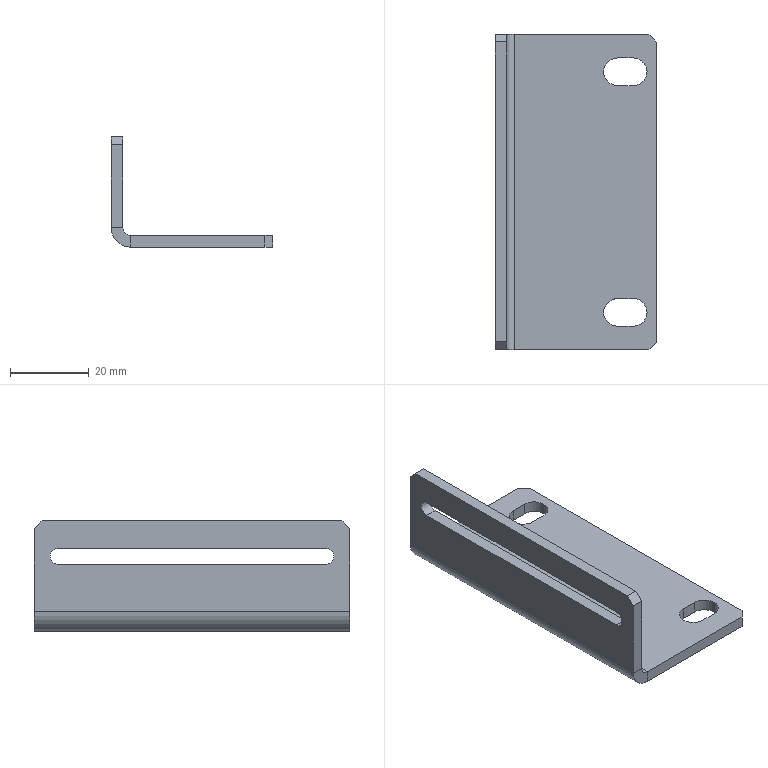Part | NX | features BREP 1 | 1 solid | 32 faces | box 41 x 80 x 28 mm | volume 14203 mm3 | plane 22 | cylinder 10 | commonest cylinder face diameters 7 x6 4 x3 10 x1
STEP:
#1=CARTESIAN_POINT('',(-2.,40.,-3.));
#2=VERTEX_POINT('',#1);
#3=CARTESIAN_POINT('',(0.,38.,-3.));
#4=VERTEX_POINT('',#3);
#5=CARTESIAN_POINT('',(0.,38.,-3.));
#6=DIRECTION('',(0.7071,-0.7071,0.));
#7=VECTOR('',#6,1000.);
#8=LINE('',#5,#7);
#9=EDGE_CURVE('',#2,#4,#8,.T.);
#10=ORIENTED_EDGE('',*,*,#9,.F.);
#11=CARTESIAN_POINT('',(-2.,40.,0.));
#12=VERTEX_POINT('',#11);
#13=CARTESIAN_POINT('',(-2.,40.,-3.));
#14=DIRECTION('',(0.,0.,-1.));
#15=VECTOR('',#14,1000.);
#16=LINE('',#13,#15);
#17=EDGE_CURVE('',#12,#2,#16,.T.);
#18=ORIENTED_EDGE('',*,*,#17,.F.);
#19=CARTESIAN_POINT('',(0.,38.,0.));
#20=VERTEX_POINT('',#19);
#21=CARTESIAN_POINT('',(-1.,39.,0.));
#22=DIRECTION('',(-0.7071,0.7071,0.));
#23=VECTOR('',#22,1000.);
#24=LINE('',#21,#23);
#25=EDGE_CURVE('',#20,#12,#24,.T.);
#26=ORIENTED_EDGE('',*,*,#25,.F.);
#27=CARTESIAN_POINT('',(0.,38.,0.));
#28=DIRECTION('',(0.,0.,1.));
#29=VECTOR('',#28,1000.);
#30=LINE('',#27,#29);
#31=EDGE_CURVE('',#4,#20,#30,.T.);
#32=ORIENTED_EDGE('',*,*,#31,.F.);
#33=EDGE_LOOP('',(#10,#18,#26,#32));
#34=FACE_BOUND('',#33,.T.);
#35=CARTESIAN_POINT('',(0.,38.,-3.));
#36=DIRECTION('',(0.7071,0.7071,0.));
#37=DIRECTION('',(0.,0.,-1.));
#38=AXIS2_PLACEMENT_3D('',#35,#36,#37);
#39=PLANE('',#38);
#40=ADVANCED_FACE('',(#34),#39,.T.);
#41=CARTESIAN_POINT('',(-38.,40.,23.));
#42=VERTEX_POINT('',#41);
#43=CARTESIAN_POINT('',(-38.,38.,25.));
#44=VERTEX_POINT('',#43);
#45=CARTESIAN_POINT('',(-38.,51.5,11.5));
#46=DIRECTION('',(0.,-0.7071,0.7071));
#47=VECTOR('',#46,1000.);
#48=LINE('',#45,#47);
#49=EDGE_CURVE('',#42,#44,#48,.T.);
#50=ORIENTED_EDGE('',*,*,#49,.F.);
#51=CARTESIAN_POINT('',(-41.,40.,23.));
#52=VERTEX_POINT('',#51);
#53=CARTESIAN_POINT('',(-36.,40.,23.));
#54=DIRECTION('',(1.,0.,0.));
#55=VECTOR('',#54,1000.);
#56=LINE('',#53,#55);
#57=EDGE_CURVE('',#52,#42,#56,.T.);
#58=ORIENTED_EDGE('',*,*,#57,.F.);
#59=CARTESIAN_POINT('',(-41.,38.,25.));
#60=VERTEX_POINT('',#59);
#61=CARTESIAN_POINT('',(-41.,38.,25.));
#62=DIRECTION('',(0.,0.7071,-0.7071));
#63=VECTOR('',#62,1000.);
#64=LINE('',#61,#63);
#65=EDGE_CURVE('',#60,#52,#64,.T.);
#66=ORIENTED_EDGE('',*,*,#65,.F.);
#67=CARTESIAN_POINT('',(-38.,38.,25.));
#68=DIRECTION('',(-1.,0.,0.));
#69=VECTOR('',#68,1000.);
#70=LINE('',#67,#69);
#71=EDGE_CURVE('',#44,#60,#70,.T.);
#72=ORIENTED_EDGE('',*,*,#71,.F.);
#73=EDGE_LOOP('',(#50,#58,#66,#72));
#74=FACE_BOUND('',#73,.T.);
#75=CARTESIAN_POINT('',(-38.,38.,25.));
#76=DIRECTION('',(0.,-0.7071,-0.7071));
#77=DIRECTION('',(-1.,0.,0.));
#78=AXIS2_PLACEMENT_3D('',#75,#76,#77);
#79=PLANE('',#78);
#80=ADVANCED_FACE('',(#74),#79,.F.);
#81=CARTESIAN_POINT('',(0.,-38.,-3.));
#82=VERTEX_POINT('',#81);
#83=CARTESIAN_POINT('',(-2.,-40.,-3.));
#84=VERTEX_POINT('',#83);
#85=CARTESIAN_POINT('',(-2.,-40.,-3.));
#86=DIRECTION('',(-0.7071,-0.7071,0.));
#87=VECTOR('',#86,1000.);
#88=LINE('',#85,#87);
#89=EDGE_CURVE('',#82,#84,#88,.T.);
#90=ORIENTED_EDGE('',*,*,#89,.F.);
#91=CARTESIAN_POINT('',(0.,-38.,0.));
#92=VERTEX_POINT('',#91);
#93=CARTESIAN_POINT('',(0.,-38.,-3.));
#94=DIRECTION('',(0.,0.,-1.));
#95=VECTOR('',#94,1000.);
#96=LINE('',#93,#95);
#97=EDGE_CURVE('',#92,#82,#96,.T.);
#98=ORIENTED_EDGE('',*,*,#97,.F.);
#99=CARTESIAN_POINT('',(-2.,-40.,0.));
#100=VERTEX_POINT('',#99);
#101=CARTESIAN_POINT('',(39.,1.,0.));
#102=DIRECTION('',(0.7071,0.7071,0.));
#103=VECTOR('',#102,1000.);
#104=LINE('',#101,#103);
#105=EDGE_CURVE('',#100,#92,#104,.T.);
#106=ORIENTED_EDGE('',*,*,#105,.F.);
#107=CARTESIAN_POINT('',(-2.,-40.,2.));
#108=DIRECTION('',(0.,0.,1.));
#109=VECTOR('',#108,1000.);
#110=LINE('',#107,#109);
#111=EDGE_CURVE('',#84,#100,#110,.T.);
#112=ORIENTED_EDGE('',*,*,#111,.F.);
#113=EDGE_LOOP('',(#90,#98,#106,#112));
#114=FACE_BOUND('',#113,.T.);
#115=CARTESIAN_POINT('',(-2.,-40.,2.));
#116=DIRECTION('',(-0.7071,0.7071,0.));
#117=DIRECTION('',(0.,0.,1.));
#118=AXIS2_PLACEMENT_3D('',#115,#116,#117);
#119=PLANE('',#118);
#120=ADVANCED_FACE('',(#114),#119,.F.);
#121=CARTESIAN_POINT('',(-38.,-38.,25.));
#122=VERTEX_POINT('',#121);
#123=CARTESIAN_POINT('',(-38.,-40.,23.));
#124=VERTEX_POINT('',#123);
#125=CARTESIAN_POINT('',(-38.,-11.5,51.5));
#126=DIRECTION('',(0.,-0.7071,-0.7071));
#127=VECTOR('',#126,1000.);
#128=LINE('',#125,#127);
#129=EDGE_CURVE('',#122,#124,#128,.T.);
#130=ORIENTED_EDGE('',*,*,#129,.F.);
#131=CARTESIAN_POINT('',(-41.,-38.,25.));
#132=VERTEX_POINT('',#131);
#133=CARTESIAN_POINT('',(-38.,-38.,25.));
#134=DIRECTION('',(1.,0.,0.));
#135=VECTOR('',#134,1000.);
#136=LINE('',#133,#135);
#137=EDGE_CURVE('',#132,#122,#136,.T.);
#138=ORIENTED_EDGE('',*,*,#137,.F.);
#139=CARTESIAN_POINT('',(-41.,-40.,23.));
#140=VERTEX_POINT('',#139);
#141=CARTESIAN_POINT('',(-41.,-40.,23.));
#142=DIRECTION('',(0.,0.7071,0.7071));
#143=VECTOR('',#142,1000.);
#144=LINE('',#141,#143);
#145=EDGE_CURVE('',#140,#132,#144,.T.);
#146=ORIENTED_EDGE('',*,*,#145,.F.);
#147=CARTESIAN_POINT('',(-36.,-40.,23.));
#148=DIRECTION('',(-1.,0.,0.));
#149=VECTOR('',#148,1000.);
#150=LINE('',#147,#149);
#151=EDGE_CURVE('',#124,#140,#150,.T.);
#152=ORIENTED_EDGE('',*,*,#151,.F.);
#153=EDGE_LOOP('',(#130,#138,#146,#152));
#154=FACE_BOUND('',#153,.T.);
#155=CARTESIAN_POINT('',(-36.,-40.,23.));
#156=DIRECTION('',(0.,0.7071,-0.7071));
#157=DIRECTION('',(-1.,0.,0.));
#158=AXIS2_PLACEMENT_3D('',#155,#156,#157);
#159=PLANE('',#158);
#160=ADVANCED_FACE('',(#154),#159,.F.);
#161=CARTESIAN_POINT('',(-10.,27.,0.));
#162=VERTEX_POINT('',#161);
#163=CARTESIAN_POINT('',(-6.,27.,0.));
#164=VERTEX_POINT('',#163);
#165=CARTESIAN_POINT('',(-10.,27.,0.));
#166=DIRECTION('',(1.,0.,0.));
#167=VECTOR('',#166,1000.);
#168=LINE('',#165,#167);
#169=EDGE_CURVE('',#162,#164,#168,.T.);
#170=ORIENTED_EDGE('',*,*,#169,.T.);
#171=CARTESIAN_POINT('',(-6.,27.,-3.));
#172=VERTEX_POINT('',#171);
#173=CARTESIAN_POINT('',(-6.,27.,-3.));
#174=DIRECTION('',(0.,0.,1.));
#175=VECTOR('',#174,1000.);
#176=LINE('',#173,#175);
#177=EDGE_CURVE('',#172,#164,#176,.T.);
#178=ORIENTED_EDGE('',*,*,#177,.F.);
#179=CARTESIAN_POINT('',(-10.,27.,-3.));
#180=VERTEX_POINT('',#179);
#181=CARTESIAN_POINT('',(-10.,27.,-3.));
#182=DIRECTION('',(1.,0.,0.));
#183=VECTOR('',#182,1000.);
#184=LINE('',#181,#183);
#185=EDGE_CURVE('',#180,#172,#184,.T.);
#186=ORIENTED_EDGE('',*,*,#185,.F.);
#187=CARTESIAN_POINT('',(-10.,27.,-3.));
#188=DIRECTION('',(0.,0.,1.));
#189=VECTOR('',#188,1000.);
#190=LINE('',#187,#189);
#191=EDGE_CURVE('',#180,#162,#190,.T.);
#192=ORIENTED_EDGE('',*,*,#191,.T.);
#193=EDGE_LOOP('',(#170,#178,#186,#192));
#194=FACE_BOUND('',#193,.T.);
#195=CARTESIAN_POINT('',(-10.,27.,-3.));
#196=DIRECTION('',(0.,-1.,0.));
#197=DIRECTION('',(0.,0.,-1.));
#198=AXIS2_PLACEMENT_3D('',#195,#196,#197);
#199=PLANE('',#198);
#200=ADVANCED_FACE('',(#194),#199,.F.);
#201=CARTESIAN_POINT('',(-2.5,30.5,-3.));
#202=VERTEX_POINT('',#201);
#203=CARTESIAN_POINT('',(-2.5,30.5,0.));
#204=VERTEX_POINT('',#203);
#205=CARTESIAN_POINT('',(-2.5,30.5,-3.));
#206=DIRECTION('',(0.,0.,1.));
#207=VECTOR('',#206,1000.);
#208=LINE('',#205,#207);
#209=EDGE_CURVE('',#202,#204,#208,.T.);
#210=ORIENTED_EDGE('',*,*,#209,.F.);
#211=CARTESIAN_POINT('',(-6.,30.5,-3.));
#212=DIRECTION('',(0.,0.,1.));
#213=DIRECTION('',(1.,0.,0.));
#214=AXIS2_PLACEMENT_3D('',#211,#212,#213);
#215=CIRCLE('',#214,3.5);
#216=EDGE_CURVE('',#172,#202,#215,.T.);
#217=ORIENTED_EDGE('',*,*,#216,.F.);
#218=ORIENTED_EDGE('',*,*,#177,.T.);
#219=CARTESIAN_POINT('',(-6.,30.5,0.));
#220=DIRECTION('',(0.,0.,1.));
#221=DIRECTION('',(1.,0.,0.));
#222=AXIS2_PLACEMENT_3D('',#219,#220,#221);
#223=CIRCLE('',#222,3.5);
#224=EDGE_CURVE('',#164,#204,#223,.T.);
#225=ORIENTED_EDGE('',*,*,#224,.T.);
#226=EDGE_LOOP('',(#210,#217,#218,#225));
#227=FACE_BOUND('',#226,.T.);
#228=CARTESIAN_POINT('',(-6.,30.5,-3.));
#229=DIRECTION('',(0.,0.,1.));
#230=DIRECTION('',(1.,0.,0.));
#231=AXIS2_PLACEMENT_3D('',#228,#229,#230);
#232=CYLINDRICAL_SURFACE('',#231,3.5);
#233=ADVANCED_FACE('',(#227),#232,.F.);
#234=CARTESIAN_POINT('',(-6.,34.,0.));
#235=VERTEX_POINT('',#234);
#236=CARTESIAN_POINT('',(-10.,34.,0.));
#237=VERTEX_POINT('',#236);
#238=CARTESIAN_POINT('',(-10.,34.,0.));
#239=DIRECTION('',(-1.,0.,0.));
#240=VECTOR('',#239,1000.);
#241=LINE('',#238,#240);
#242=EDGE_CURVE('',#235,#237,#241,.T.);
#243=ORIENTED_EDGE('',*,*,#242,.T.);
#244=CARTESIAN_POINT('',(-10.,34.,-3.));
#245=VERTEX_POINT('',#244);
#246=CARTESIAN_POINT('',(-10.,34.,-3.));
#247=DIRECTION('',(0.,0.,1.));
#248=VECTOR('',#247,1000.);
#249=LINE('',#246,#248);
#250=EDGE_CURVE('',#245,#237,#249,.T.);
#251=ORIENTED_EDGE('',*,*,#250,.F.);
#252=CARTESIAN_POINT('',(-6.,34.,-3.));
#253=VERTEX_POINT('',#252);
#254=CARTESIAN_POINT('',(-10.,34.,-3.));
#255=DIRECTION('',(-1.,0.,0.));
#256=VECTOR('',#255,1000.);
#257=LINE('',#254,#256);
#258=EDGE_CURVE('',#253,#245,#257,.T.);
#259=ORIENTED_EDGE('',*,*,#258,.F.);
#260=CARTESIAN_POINT('',(-6.,34.,-3.));
#261=DIRECTION('',(0.,0.,1.));
#262=VECTOR('',#261,1000.);
#263=LINE('',#260,#262);
#264=EDGE_CURVE('',#253,#235,#263,.T.);
#265=ORIENTED_EDGE('',*,*,#264,.T.);
#266=EDGE_LOOP('',(#243,#251,#259,#265));
#267=FACE_BOUND('',#266,.T.);
#268=CARTESIAN_POINT('',(-10.,34.,-3.));
#269=DIRECTION('',(0.,1.,0.));
#270=DIRECTION('',(0.,0.,1.));
#271=AXIS2_PLACEMENT_3D('',#268,#269,#270);
#272=PLANE('',#271);
#273=ADVANCED_FACE('',(#267),#272,.F.);
#274=CARTESIAN_POINT('',(-10.,30.5,0.));
#275=DIRECTION('',(0.,0.,1.));
#276=DIRECTION('',(1.,0.,0.));
#277=AXIS2_PLACEMENT_3D('',#274,#275,#276);
#278=CIRCLE('',#277,3.5);
#279=EDGE_CURVE('',#237,#162,#278,.T.);
#280=ORIENTED_EDGE('',*,*,#279,.T.);
#281=ORIENTED_EDGE('',*,*,#191,.F.);
#282=CARTESIAN_POINT('',(-10.,30.5,-3.));
#283=DIRECTION('',(0.,0.,1.));
#284=DIRECTION('',(1.,0.,0.));
#285=AXIS2_PLACEMENT_3D('',#282,#283,#284);
#286=CIRCLE('',#285,3.5);
#287=EDGE_CURVE('',#245,#180,#286,.T.);
#288=ORIENTED_EDGE('',*,*,#287,.F.);
#289=ORIENTED_EDGE('',*,*,#250,.T.);
#290=EDGE_LOOP('',(#280,#281,#288,#289));
#291=FACE_BOUND('',#290,.T.);
#292=CARTESIAN_POINT('',(-10.,30.5,-3.));
#293=DIRECTION('',(0.,0.,1.));
#294=DIRECTION('',(1.,0.,0.));
#295=AXIS2_PLACEMENT_3D('',#292,#293,#294);
#296=CYLINDRICAL_SURFACE('',#295,3.5);
#297=ADVANCED_FACE('',(#291),#296,.F.);
#298=CARTESIAN_POINT('',(-6.,-27.,0.));
#299=VERTEX_POINT('',#298);
#300=CARTESIAN_POINT('',(-10.,-27.,0.));
#301=VERTEX_POINT('',#300);
#302=CARTESIAN_POINT('',(-6.,-27.,0.));
#303=DIRECTION('',(-1.,0.,0.));
#304=VECTOR('',#303,1000.);
#305=LINE('',#302,#304);
#306=EDGE_CURVE('',#299,#301,#305,.T.);
#307=ORIENTED_EDGE('',*,*,#306,.T.);
#308=CARTESIAN_POINT('',(-10.,-27.,-3.));
#309=VERTEX_POINT('',#308);
#310=CARTESIAN_POINT('',(-10.,-27.,-3.));
#311=DIRECTION('',(0.,0.,1.));
#312=VECTOR('',#311,1000.);
#313=LINE('',#310,#312);
#314=EDGE_CURVE('',#309,#301,#313,.T.);
#315=ORIENTED_EDGE('',*,*,#314,.F.);
#316=CARTESIAN_POINT('',(-6.,-27.,-3.));
#317=VERTEX_POINT('',#316);
#318=CARTESIAN_POINT('',(-6.,-27.,-3.));
#319=DIRECTION('',(-1.,0.,0.));
#320=VECTOR('',#319,1000.);
#321=LINE('',#318,#320);
#322=EDGE_CURVE('',#317,#309,#321,.T.);
#323=ORIENTED_EDGE('',*,*,#322,.F.);
#324=CARTESIAN_POINT('',(-6.,-27.,-3.));
#325=DIRECTION('',(0.,0.,1.));
#326=VECTOR('',#325,1000.);
#327=LINE('',#324,#326);
#328=EDGE_CURVE('',#317,#299,#327,.T.);
#329=ORIENTED_EDGE('',*,*,#328,.T.);
#330=EDGE_LOOP('',(#307,#315,#323,#329));
#331=FACE_BOUND('',#330,.T.);
#332=CARTESIAN_POINT('',(-6.,-27.,-3.));
#333=DIRECTION('',(0.,1.,0.));
#334=DIRECTION('',(0.,0.,1.));
#335=AXIS2_PLACEMENT_3D('',#332,#333,#334);
#336=PLANE('',#335);
#337=ADVANCED_FACE('',(#331),#336,.F.);
#338=CARTESIAN_POINT('',(-10.,-34.,0.));
#339=VERTEX_POINT('',#338);
#340=CARTESIAN_POINT('',(-10.,-30.5,0.));
#341=DIRECTION('',(0.,0.,1.));
#342=DIRECTION('',(1.,0.,0.));
#343=AXIS2_PLACEMENT_3D('',#340,#341,#342);
#344=CIRCLE('',#343,3.5);
#345=EDGE_CURVE('',#301,#339,#344,.T.);
#346=ORIENTED_EDGE('',*,*,#345,.T.);
#347=CARTESIAN_POINT('',(-10.,-34.,-3.));
#348=VERTEX_POINT('',#347);
#349=CARTESIAN_POINT('',(-10.,-34.,-3.));
#350=DIRECTION('',(0.,0.,1.));
#351=VECTOR('',#350,1000.);
#352=LINE('',#349,#351);
#353=EDGE_CURVE('',#348,#339,#352,.T.);
#354=ORIENTED_EDGE('',*,*,#353,.F.);
#355=CARTESIAN_POINT('',(-10.,-30.5,-3.));
#356=DIRECTION('',(0.,0.,1.));
#357=DIRECTION('',(1.,0.,0.));
#358=AXIS2_PLACEMENT_3D('',#355,#356,#357);
#359=CIRCLE('',#358,3.5);
#360=EDGE_CURVE('',#309,#348,#359,.T.);
#361=ORIENTED_EDGE('',*,*,#360,.F.);
#362=ORIENTED_EDGE('',*,*,#314,.T.);
#363=EDGE_LOOP('',(#346,#354,#361,#362));
#364=FACE_BOUND('',#363,.T.);
#365=CARTESIAN_POINT('',(-10.,-30.5,-3.));
#366=DIRECTION('',(0.,0.,1.));
#367=DIRECTION('',(1.,0.,0.));
#368=AXIS2_PLACEMENT_3D('',#365,#366,#367);
#369=CYLINDRICAL_SURFACE('',#368,3.5);
#370=ADVANCED_FACE('',(#364),#369,.F.);
#371=CARTESIAN_POINT('',(-6.,-34.,0.));
#372=VERTEX_POINT('',#371);
#373=CARTESIAN_POINT('',(-6.,-34.,0.));
#374=DIRECTION('',(1.,0.,0.));
#375=VECTOR('',#374,1000.);
#376=LINE('',#373,#375);
#377=EDGE_CURVE('',#339,#372,#376,.T.);
#378=ORIENTED_EDGE('',*,*,#377,.T.);
#379=CARTESIAN_POINT('',(-6.,-34.,-3.));
#380=VERTEX_POINT('',#379);
#381=CARTESIAN_POINT('',(-6.,-34.,-3.));
#382=DIRECTION('',(0.,0.,1.));
#383=VECTOR('',#382,1000.);
#384=LINE('',#381,#383);
#385=EDGE_CURVE('',#380,#372,#384,.T.);
#386=ORIENTED_EDGE('',*,*,#385,.F.);
#387=CARTESIAN_POINT('',(-6.,-34.,-3.));
#388=DIRECTION('',(1.,0.,0.));
#389=VECTOR('',#388,1000.);
#390=LINE('',#387,#389);
#391=EDGE_CURVE('',#348,#380,#390,.T.);
#392=ORIENTED_EDGE('',*,*,#391,.F.);
#393=ORIENTED_EDGE('',*,*,#353,.T.);
#394=EDGE_LOOP('',(#378,#386,#392,#393));
#395=FACE_BOUND('',#394,.T.);
#396=CARTESIAN_POINT('',(-6.,-34.,-3.));
#397=DIRECTION('',(0.,-1.,0.));
#398=DIRECTION('',(0.,0.,-1.));
#399=AXIS2_PLACEMENT_3D('',#396,#397,#398);
#400=PLANE('',#399);
#401=ADVANCED_FACE('',(#395),#400,.F.);
#402=CARTESIAN_POINT('',(-2.5,-30.5,-3.));
#403=VERTEX_POINT('',#402);
#404=CARTESIAN_POINT('',(-2.5,-30.5,0.));
#405=VERTEX_POINT('',#404);
#406=CARTESIAN_POINT('',(-2.5,-30.5,-3.));
#407=DIRECTION('',(0.,0.,1.));
#408=VECTOR('',#407,1000.);
#409=LINE('',#406,#408);
#410=EDGE_CURVE('',#403,#405,#409,.T.);
#411=ORIENTED_EDGE('',*,*,#410,.F.);
#412=CARTESIAN_POINT('',(-6.,-30.5,-3.));
#413=DIRECTION('',(0.,0.,1.));
#414=DIRECTION('',(1.,0.,0.));
#415=AXIS2_PLACEMENT_3D('',#412,#413,#414);
#416=CIRCLE('',#415,3.5);
#417=EDGE_CURVE('',#380,#403,#416,.T.);
#418=ORIENTED_EDGE('',*,*,#417,.F.);
#419=ORIENTED_EDGE('',*,*,#385,.T.);
#420=CARTESIAN_POINT('',(-6.,-30.5,0.));
#421=DIRECTION('',(0.,0.,1.));
#422=DIRECTION('',(1.,0.,0.));
#423=AXIS2_PLACEMENT_3D('',#420,#421,#422);
#424=CIRCLE('',#423,3.5);
#425=EDGE_CURVE('',#372,#405,#424,.T.);
#426=ORIENTED_EDGE('',*,*,#425,.T.);
#427=EDGE_LOOP('',(#411,#418,#419,#426));
#428=FACE_BOUND('',#427,.T.);
#429=CARTESIAN_POINT('',(-6.,-30.5,-3.));
#430=DIRECTION('',(0.,0.,1.));
#431=DIRECTION('',(1.,0.,0.));
#432=AXIS2_PLACEMENT_3D('',#429,#430,#431);
#433=CYLINDRICAL_SURFACE('',#432,3.5);
#434=ADVANCED_FACE('',(#428),#433,.F.);
#435=CARTESIAN_POINT('',(-38.,34.,18.));
#436=VERTEX_POINT('',#435);
#437=CARTESIAN_POINT('',(-38.,-34.,18.));
#438=VERTEX_POINT('',#437);
#439=CARTESIAN_POINT('',(-38.,34.,18.));
#440=DIRECTION('',(0.,-1.,0.));
#441=VECTOR('',#440,1000.);
#442=LINE('',#439,#441);
#443=EDGE_CURVE('',#436,#438,#442,.T.);
#444=ORIENTED_EDGE('',*,*,#443,.T.);
#445=CARTESIAN_POINT('',(-41.,-34.,18.));
#446=VERTEX_POINT('',#445);
#447=CARTESIAN_POINT('',(-41.,-34.,18.));
#448=DIRECTION('',(1.,0.,0.));
#449=VECTOR('',#448,1000.);
#450=LINE('',#447,#449);
#451=EDGE_CURVE('',#446,#438,#450,.T.);
#452=ORIENTED_EDGE('',*,*,#451,.F.);
#453=CARTESIAN_POINT('',(-41.,34.,18.));
#454=VERTEX_POINT('',#453);
#455=CARTESIAN_POINT('',(-41.,34.,18.));
#456=DIRECTION('',(0.,-1.,0.));
#457=VECTOR('',#456,1000.);
#458=LINE('',#455,#457);
#459=EDGE_CURVE('',#454,#446,#458,.T.);
#460=ORIENTED_EDGE('',*,*,#459,.F.);
#461=CARTESIAN_POINT('',(-41.,34.,18.));
#462=DIRECTION('',(1.,0.,0.));
#463=VECTOR('',#462,1000.);
#464=LINE('',#461,#463);
#465=EDGE_CURVE('',#454,#436,#464,.T.);
#466=ORIENTED_EDGE('',*,*,#465,.T.);
#467=EDGE_LOOP('',(#444,#452,#460,#466));
#468=FACE_BOUND('',#467,.T.);
#469=CARTESIAN_POINT('',(-41.,34.,18.));
#470=DIRECTION('',(0.,0.,1.));
#471=DIRECTION('',(1.,0.,0.));
#472=AXIS2_PLACEMENT_3D('',#469,#470,#471);
#473=PLANE('',#472);
#474=ADVANCED_FACE('',(#468),#473,.F.);
#475=CARTESIAN_POINT('',(-38.,-34.,14.));
#476=VERTEX_POINT('',#475);
#477=CARTESIAN_POINT('',(-38.,-34.,16.));
#478=DIRECTION('',(1.,0.,0.));
#479=DIRECTION('',(0.,0.,-1.));
#480=AXIS2_PLACEMENT_3D('',#477,#478,#479);
#481=CIRCLE('',#480,2.);
#482=EDGE_CURVE('',#438,#476,#481,.T.);
#483=ORIENTED_EDGE('',*,*,#482,.T.);
#484=CARTESIAN_POINT('',(-41.,-34.,14.));
#485=VERTEX_POINT('',#484);
#486=CARTESIAN_POINT('',(-41.,-34.,14.));
#487=DIRECTION('',(1.,0.,0.));
#488=VECTOR('',#487,1000.);
#489=LINE('',#486,#488);
#490=EDGE_CURVE('',#485,#476,#489,.T.);
#491=ORIENTED_EDGE('',*,*,#490,.F.);
#492=CARTESIAN_POINT('',(-41.,-34.,16.));
#493=DIRECTION('',(1.,0.,0.));
#494=DIRECTION('',(0.,0.,-1.));
#495=AXIS2_PLACEMENT_3D('',#492,#493,#494);
#496=CIRCLE('',#495,2.);
#497=EDGE_CURVE('',#446,#485,#496,.T.);
#498=ORIENTED_EDGE('',*,*,#497,.F.);
#499=ORIENTED_EDGE('',*,*,#451,.T.);
#500=EDGE_LOOP('',(#483,#491,#498,#499));
#501=FACE_BOUND('',#500,.T.);
#502=CARTESIAN_POINT('',(-41.,-34.,16.));
#503=DIRECTION('',(1.,0.,0.));
#504=DIRECTION('',(0.,0.,-1.));
#505=AXIS2_PLACEMENT_3D('',#502,#503,#504);
#506=CYLINDRICAL_SURFACE('',#505,2.);
#507=ADVANCED_FACE('',(#501),#506,.F.);
#508=CARTESIAN_POINT('',(-38.,34.,14.));
#509=VERTEX_POINT('',#508);
#510=CARTESIAN_POINT('',(-38.,34.,14.));
#511=DIRECTION('',(0.,1.,0.));
#512=VECTOR('',#511,1000.);
#513=LINE('',#510,#512);
#514=EDGE_CURVE('',#476,#509,#513,.T.);
#515=ORIENTED_EDGE('',*,*,#514,.T.);
#516=CARTESIAN_POINT('',(-41.,34.,14.));
#517=VERTEX_POINT('',#516);
#518=CARTESIAN_POINT('',(-41.,34.,14.));
#519=DIRECTION('',(1.,0.,0.));
#520=VECTOR('',#519,1000.);
#521=LINE('',#518,#520);
#522=EDGE_CURVE('',#517,#509,#521,.T.);
#523=ORIENTED_EDGE('',*,*,#522,.F.);
#524=CARTESIAN_POINT('',(-41.,34.,14.));
#525=DIRECTION('',(0.,1.,0.));
#526=VECTOR('',#525,1000.);
#527=LINE('',#524,#526);
#528=EDGE_CURVE('',#485,#517,#527,.T.);
#529=ORIENTED_EDGE('',*,*,#528,.F.);
#530=ORIENTED_EDGE('',*,*,#490,.T.);
#531=EDGE_LOOP('',(#515,#523,#529,#530));
#532=FACE_BOUND('',#531,.T.);
#533=CARTESIAN_POINT('',(-41.,34.,14.));
#534=DIRECTION('',(0.,0.,-1.));
#535=DIRECTION('',(-1.,0.,0.));
#536=AXIS2_PLACEMENT_3D('',#533,#534,#535);
#537=PLANE('',#536);
#538=ADVANCED_FACE('',(#532),#537,.F.);
#539=CARTESIAN_POINT('',(-38.,34.,16.));
#540=DIRECTION('',(1.,0.,0.));
#541=DIRECTION('',(0.,0.,-1.));
#542=AXIS2_PLACEMENT_3D('',#539,#540,#541);
#543=CIRCLE('',#542,2.);
#544=EDGE_CURVE('',#509,#436,#543,.T.);
#545=ORIENTED_EDGE('',*,*,#544,.T.);
#546=ORIENTED_EDGE('',*,*,#465,.F.);
#547=CARTESIAN_POINT('',(-41.,34.,16.));
#548=DIRECTION('',(1.,0.,0.));
#549=DIRECTION('',(0.,0.,-1.));
#550=AXIS2_PLACEMENT_3D('',#547,#548,#549);
#551=CIRCLE('',#550,2.);
#552=EDGE_CURVE('',#517,#454,#551,.T.);
#553=ORIENTED_EDGE('',*,*,#552,.F.);
#554=ORIENTED_EDGE('',*,*,#522,.T.);
#555=EDGE_LOOP('',(#545,#546,#553,#554));
#556=FACE_BOUND('',#555,.T.);
#557=CARTESIAN_POINT('',(-41.,34.,16.));
#558=DIRECTION('',(1.,0.,0.));
#559=DIRECTION('',(0.,0.,-1.));
#560=AXIS2_PLACEMENT_3D('',#557,#558,#559);
#561=CYLINDRICAL_SURFACE('',#560,2.);
#562=ADVANCED_FACE('',(#556),#561,.F.);
#563=CARTESIAN_POINT('',(-38.,-40.,2.));
#564=VERTEX_POINT('',#563);
#565=CARTESIAN_POINT('',(-38.,-40.,0.));
#566=DIRECTION('',(0.,0.,1.));
#567=VECTOR('',#566,1000.);
#568=LINE('',#565,#567);
#569=EDGE_CURVE('',#564,#124,#568,.T.);
#570=ORIENTED_EDGE('',*,*,#569,.T.);
#571=ORIENTED_EDGE('',*,*,#151,.T.);
#572=CARTESIAN_POINT('',(-41.,-40.,2.));
#573=VERTEX_POINT('',#572);
#574=CARTESIAN_POINT('',(-41.,-40.,0.));
#575=DIRECTION('',(0.,0.,1.));
#576=VECTOR('',#575,1000.);
#577=LINE('',#574,#576);
#578=EDGE_CURVE('',#573,#140,#577,.T.);
#579=ORIENTED_EDGE('',*,*,#578,.F.);
#580=CARTESIAN_POINT('',(-41.,-40.,2.));
#581=DIRECTION('',(1.,0.,0.));
#582=VECTOR('',#581,1000.);
#583=LINE('',#580,#582);
#584=EDGE_CURVE('',#573,#564,#583,.T.);
#585=ORIENTED_EDGE('',*,*,#584,.T.);
#586=EDGE_LOOP('',(#570,#571,#579,#585));
#587=FACE_BOUND('',#586,.T.);
#588=CARTESIAN_POINT('',(-36.,-40.,2.));
#589=DIRECTION('',(0.,-1.,0.));
#590=DIRECTION('',(-1.,0.,0.));
#591=AXIS2_PLACEMENT_3D('',#588,#589,#590);
#592=PLANE('',#591);
#593=ADVANCED_FACE('',(#587),#592,.T.);
#594=CARTESIAN_POINT('',(-36.,40.,0.));
#595=VERTEX_POINT('',#594);
#596=CARTESIAN_POINT('',(0.,40.,0.));
#597=DIRECTION('',(-1.,0.,0.));
#598=VECTOR('',#597,1000.);
#599=LINE('',#596,#598);
#600=EDGE_CURVE('',#12,#595,#599,.T.);
#601=ORIENTED_EDGE('',*,*,#600,.F.);
#602=ORIENTED_EDGE('',*,*,#17,.T.);
#603=CARTESIAN_POINT('',(-36.,40.,-3.));
#604=VERTEX_POINT('',#603);
#605=CARTESIAN_POINT('',(0.,40.,-3.));
#606=DIRECTION('',(-1.,0.,0.));
#607=VECTOR('',#606,1000.);
#608=LINE('',#605,#607);
#609=EDGE_CURVE('',#2,#604,#608,.T.);
#610=ORIENTED_EDGE('',*,*,#609,.T.);
#611=CARTESIAN_POINT('',(-36.,40.,-3.));
#612=DIRECTION('',(0.,0.,1.));
#613=VECTOR('',#612,1000.);
#614=LINE('',#611,#613);
#615=EDGE_CURVE('',#604,#595,#614,.T.);
#616=ORIENTED_EDGE('',*,*,#615,.T.);
#617=EDGE_LOOP('',(#601,#602,#610,#616));
#618=FACE_BOUND('',#617,.T.);
#619=CARTESIAN_POINT('',(-36.,40.,2.));
#620=DIRECTION('',(0.,-1.,0.));
#621=DIRECTION('',(-1.,0.,0.));
#622=AXIS2_PLACEMENT_3D('',#619,#620,#621);
#623=PLANE('',#622);
#624=ADVANCED_FACE('',(#618),#623,.F.);
#625=CARTESIAN_POINT('',(-36.,-40.,-3.));
#626=VERTEX_POINT('',#625);
#627=CARTESIAN_POINT('',(-36.,-40.,2.));
#628=DIRECTION('',(0.,1.,0.));
#629=DIRECTION('',(1.,0.,0.));
#630=AXIS2_PLACEMENT_3D('',#627,#628,#629);
#631=CIRCLE('',#630,5.);
#632=EDGE_CURVE('',#626,#573,#631,.T.);
#633=ORIENTED_EDGE('',*,*,#632,.T.);
#634=CARTESIAN_POINT('',(-41.,40.,2.));
#635=VERTEX_POINT('',#634);
#636=CARTESIAN_POINT('',(-41.,40.,2.));
#637=DIRECTION('',(0.,-1.,0.));
#638=VECTOR('',#637,1000.);
#639=LINE('',#636,#638);
#640=EDGE_CURVE('',#635,#573,#639,.T.);
#641=ORIENTED_EDGE('',*,*,#640,.F.);
#642=CARTESIAN_POINT('',(-36.,40.,2.));
#643=DIRECTION('',(0.,1.,0.));
#644=DIRECTION('',(1.,0.,0.));
#645=AXIS2_PLACEMENT_3D('',#642,#643,#644);
#646=CIRCLE('',#645,5.);
#647=EDGE_CURVE('',#604,#635,#646,.T.);
#648=ORIENTED_EDGE('',*,*,#647,.F.);
#649=CARTESIAN_POINT('',(-36.,40.,-3.));
#650=DIRECTION('',(0.,-1.,0.));
#651=VECTOR('',#650,1000.);
#652=LINE('',#649,#651);
#653=EDGE_CURVE('',#604,#626,#652,.T.);
#654=ORIENTED_EDGE('',*,*,#653,.T.);
#655=EDGE_LOOP('',(#633,#641,#648,#654));
#656=FACE_BOUND('',#655,.T.);
#657=CARTESIAN_POINT('',(-36.,40.,2.));
#658=DIRECTION('',(0.,-1.,0.));
#659=DIRECTION('',(0.,0.,-1.));
#660=AXIS2_PLACEMENT_3D('',#657,#658,#659);
#661=CYLINDRICAL_SURFACE('',#660,5.);
#662=ADVANCED_FACE('',(#656),#661,.T.);
#663=CARTESIAN_POINT('',(0.,40.,-3.));
#664=DIRECTION('',(0.,-1.,0.));
#665=VECTOR('',#664,1000.);
#666=LINE('',#663,#665);
#667=EDGE_CURVE('',#4,#82,#666,.T.);
#668=ORIENTED_EDGE('',*,*,#667,.T.);
#669=ORIENTED_EDGE('',*,*,#89,.T.);
#670=CARTESIAN_POINT('',(0.,-40.,-3.));
#671=DIRECTION('',(-1.,0.,0.));
#672=VECTOR('',#671,1000.);
#673=LINE('',#670,#672);
#674=EDGE_CURVE('',#84,#626,#673,.T.);
#675=ORIENTED_EDGE('',*,*,#674,.T.);
#676=ORIENTED_EDGE('',*,*,#653,.F.);
#677=ORIENTED_EDGE('',*,*,#609,.F.);
#678=ORIENTED_EDGE('',*,*,#9,.T.);
#679=EDGE_LOOP('',(#668,#669,#675,#676,#677,#678));
#680=FACE_BOUND('',#679,.T.);
#681=ORIENTED_EDGE('',*,*,#391,.T.);
#682=ORIENTED_EDGE('',*,*,#417,.T.);
#683=CARTESIAN_POINT('',(-6.,-30.5,-3.));
#684=DIRECTION('',(0.,0.,1.));
#685=DIRECTION('',(1.,0.,0.));
#686=AXIS2_PLACEMENT_3D('',#683,#684,#685);
#687=CIRCLE('',#686,3.5);
#688=EDGE_CURVE('',#403,#317,#687,.T.);
#689=ORIENTED_EDGE('',*,*,#688,.T.);
#690=ORIENTED_EDGE('',*,*,#322,.T.);
#691=ORIENTED_EDGE('',*,*,#360,.T.);
#692=EDGE_LOOP('',(#681,#682,#689,#690,#691));
#693=FACE_BOUND('',#692,.T.);
#694=ORIENTED_EDGE('',*,*,#258,.T.);
#695=ORIENTED_EDGE('',*,*,#287,.T.);
#696=ORIENTED_EDGE('',*,*,#185,.T.);
#697=ORIENTED_EDGE('',*,*,#216,.T.);
#698=CARTESIAN_POINT('',(-6.,30.5,-3.));
#699=DIRECTION('',(0.,0.,1.));
#700=DIRECTION('',(1.,0.,0.));
#701=AXIS2_PLACEMENT_3D('',#698,#699,#700);
#702=CIRCLE('',#701,3.5);
#703=EDGE_CURVE('',#202,#253,#702,.T.);
#704=ORIENTED_EDGE('',*,*,#703,.T.);
#705=EDGE_LOOP('',(#694,#695,#696,#697,#704));
#706=FACE_BOUND('',#705,.T.);
#707=CARTESIAN_POINT('',(0.,40.,-3.));
#708=DIRECTION('',(0.,0.,1.));
#709=DIRECTION('',(1.,0.,0.));
#710=AXIS2_PLACEMENT_3D('',#707,#708,#709);
#711=PLANE('',#710);
#712=ADVANCED_FACE('',(#680,#693,#706),#711,.F.);
#713=CARTESIAN_POINT('',(0.,40.,0.));
#714=DIRECTION('',(0.,-1.,0.));
#715=VECTOR('',#714,1000.);
#716=LINE('',#713,#715);
#717=EDGE_CURVE('',#20,#92,#716,.T.);
#718=ORIENTED_EDGE('',*,*,#717,.T.);
#719=ORIENTED_EDGE('',*,*,#97,.T.);
#720=ORIENTED_EDGE('',*,*,#667,.F.);
#721=ORIENTED_EDGE('',*,*,#31,.T.);
#722=EDGE_LOOP('',(#718,#719,#720,#721));
#723=FACE_BOUND('',#722,.T.);
#724=CARTESIAN_POINT('',(0.,40.,-3.));
#725=DIRECTION('',(1.,0.,0.));
#726=DIRECTION('',(0.,0.,-1.));
#727=AXIS2_PLACEMENT_3D('',#724,#725,#726);
#728=PLANE('',#727);
#729=ADVANCED_FACE('',(#723),#728,.T.);
#730=CARTESIAN_POINT('',(-36.,-40.,0.));
#731=VERTEX_POINT('',#730);
#732=CARTESIAN_POINT('',(0.,-40.,0.));
#733=DIRECTION('',(-1.,0.,0.));
#734=VECTOR('',#733,1000.);
#735=LINE('',#732,#734);
#736=EDGE_CURVE('',#100,#731,#735,.T.);
#737=ORIENTED_EDGE('',*,*,#736,.F.);
#738=ORIENTED_EDGE('',*,*,#105,.T.);
#739=ORIENTED_EDGE('',*,*,#717,.F.);
#740=ORIENTED_EDGE('',*,*,#25,.T.);
#741=ORIENTED_EDGE('',*,*,#600,.T.);
#742=CARTESIAN_POINT('',(-36.,40.,0.));
#743=DIRECTION('',(0.,-1.,0.));
#744=VECTOR('',#743,1000.);
#745=LINE('',#742,#744);
#746=EDGE_CURVE('',#595,#731,#745,.T.);
#747=ORIENTED_EDGE('',*,*,#746,.T.);
#748=EDGE_LOOP('',(#737,#738,#739,#740,#741,#747));
#749=FACE_BOUND('',#748,.T.);
#750=ORIENTED_EDGE('',*,*,#425,.F.);
#751=ORIENTED_EDGE('',*,*,#377,.F.);
#752=ORIENTED_EDGE('',*,*,#345,.F.);
#753=ORIENTED_EDGE('',*,*,#306,.F.);
#754=CARTESIAN_POINT('',(-6.,-30.5,0.));
#755=DIRECTION('',(0.,0.,1.));
#756=DIRECTION('',(1.,0.,0.));
#757=AXIS2_PLACEMENT_3D('',#754,#755,#756);
#758=CIRCLE('',#757,3.5);
#759=EDGE_CURVE('',#405,#299,#758,.T.);
#760=ORIENTED_EDGE('',*,*,#759,.F.);
#761=EDGE_LOOP('',(#750,#751,#752,#753,#760));
#762=FACE_BOUND('',#761,.T.);
#763=ORIENTED_EDGE('',*,*,#279,.F.);
#764=ORIENTED_EDGE('',*,*,#242,.F.);
#765=CARTESIAN_POINT('',(-6.,30.5,0.));
#766=DIRECTION('',(0.,0.,1.));
#767=DIRECTION('',(1.,0.,0.));
#768=AXIS2_PLACEMENT_3D('',#765,#766,#767);
#769=CIRCLE('',#768,3.5);
#770=EDGE_CURVE('',#204,#235,#769,.T.);
#771=ORIENTED_EDGE('',*,*,#770,.F.);
#772=ORIENTED_EDGE('',*,*,#224,.F.);
#773=ORIENTED_EDGE('',*,*,#169,.F.);
#774=EDGE_LOOP('',(#763,#764,#771,#772,#773));
#775=FACE_BOUND('',#774,.T.);
#776=CARTESIAN_POINT('',(0.,40.,0.));
#777=DIRECTION('',(0.,0.,1.));
#778=DIRECTION('',(1.,0.,0.));
#779=AXIS2_PLACEMENT_3D('',#776,#777,#778);
#780=PLANE('',#779);
#781=ADVANCED_FACE('',(#749,#762,#775),#780,.T.);
#782=CARTESIAN_POINT('',(-36.,-40.,2.));
#783=DIRECTION('',(0.,1.,0.));
#784=DIRECTION('',(0.,0.,-1.));
#785=AXIS2_PLACEMENT_3D('',#782,#783,#784);
#786=CIRCLE('',#785,2.);
#787=EDGE_CURVE('',#731,#564,#786,.T.);
#788=ORIENTED_EDGE('',*,*,#787,.F.);
#789=ORIENTED_EDGE('',*,*,#746,.F.);
#790=CARTESIAN_POINT('',(-38.,40.,2.));
#791=VERTEX_POINT('',#790);
#792=CARTESIAN_POINT('',(-36.,40.,2.));
#793=DIRECTION('',(0.,1.,0.));
#794=DIRECTION('',(0.,0.,-1.));
#795=AXIS2_PLACEMENT_3D('',#792,#793,#794);
#796=CIRCLE('',#795,2.);
#797=EDGE_CURVE('',#595,#791,#796,.T.);
#798=ORIENTED_EDGE('',*,*,#797,.T.);
#799=CARTESIAN_POINT('',(-38.,40.,2.));
#800=DIRECTION('',(0.,-1.,0.));
#801=VECTOR('',#800,1000.);
#802=LINE('',#799,#801);
#803=EDGE_CURVE('',#791,#564,#802,.T.);
#804=ORIENTED_EDGE('',*,*,#803,.T.);
#805=EDGE_LOOP('',(#788,#789,#798,#804));
#806=FACE_BOUND('',#805,.T.);
#807=CARTESIAN_POINT('',(-36.,40.,2.));
#808=DIRECTION('',(0.,-1.,0.));
#809=DIRECTION('',(0.,0.,-1.));
#810=AXIS2_PLACEMENT_3D('',#807,#808,#809);
#811=CYLINDRICAL_SURFACE('',#810,2.);
#812=ADVANCED_FACE('',(#806),#811,.F.);
#813=CARTESIAN_POINT('',(-38.,40.,25.));
#814=DIRECTION('',(0.,-1.,0.));
#815=VECTOR('',#814,1000.);
#816=LINE('',#813,#815);
#817=EDGE_CURVE('',#44,#122,#816,.T.);
#818=ORIENTED_EDGE('',*,*,#817,.T.);
#819=ORIENTED_EDGE('',*,*,#129,.T.);
#820=ORIENTED_EDGE('',*,*,#569,.F.);
#821=ORIENTED_EDGE('',*,*,#803,.F.);
#822=CARTESIAN_POINT('',(-38.,40.,0.));
#823=DIRECTION('',(0.,0.,1.));
#824=VECTOR('',#823,1000.);
#825=LINE('',#822,#824);
#826=EDGE_CURVE('',#791,#42,#825,.T.);
#827=ORIENTED_EDGE('',*,*,#826,.T.);
#828=ORIENTED_EDGE('',*,*,#49,.T.);
#829=EDGE_LOOP('',(#818,#819,#820,#821,#827,#828));
#830=FACE_BOUND('',#829,.T.);
#831=ORIENTED_EDGE('',*,*,#544,.F.);
#832=ORIENTED_EDGE('',*,*,#514,.F.);
#833=ORIENTED_EDGE('',*,*,#482,.F.);
#834=ORIENTED_EDGE('',*,*,#443,.F.);
#835=EDGE_LOOP('',(#831,#832,#833,#834));
#836=FACE_BOUND('',#835,.T.);
#837=CARTESIAN_POINT('',(-38.,40.,0.));
#838=DIRECTION('',(1.,0.,0.));
#839=DIRECTION('',(0.,0.,-1.));
#840=AXIS2_PLACEMENT_3D('',#837,#838,#839);
#841=PLANE('',#840);
#842=ADVANCED_FACE('',(#830,#836),#841,.T.);
#843=CARTESIAN_POINT('',(-41.,40.,25.));
#844=DIRECTION('',(0.,-1.,0.));
#845=VECTOR('',#844,1000.);
#846=LINE('',#843,#845);
#847=EDGE_CURVE('',#60,#132,#846,.T.);
#848=ORIENTED_EDGE('',*,*,#847,.T.);
#849=ORIENTED_EDGE('',*,*,#137,.T.);
#850=ORIENTED_EDGE('',*,*,#817,.F.);
#851=ORIENTED_EDGE('',*,*,#71,.T.);
#852=EDGE_LOOP('',(#848,#849,#850,#851));
#853=FACE_BOUND('',#852,.T.);
#854=CARTESIAN_POINT('',(-38.,40.,25.));
#855=DIRECTION('',(0.,0.,1.));
#856=DIRECTION('',(1.,0.,0.));
#857=AXIS2_PLACEMENT_3D('',#854,#855,#856);
#858=PLANE('',#857);
#859=ADVANCED_FACE('',(#853),#858,.T.);
#860=ORIENTED_EDGE('',*,*,#578,.T.);
#861=ORIENTED_EDGE('',*,*,#145,.T.);
#862=ORIENTED_EDGE('',*,*,#847,.F.);
#863=ORIENTED_EDGE('',*,*,#65,.T.);
#864=CARTESIAN_POINT('',(-41.,40.,0.));
#865=DIRECTION('',(0.,0.,1.));
#866=VECTOR('',#865,1000.);
#867=LINE('',#864,#866);
#868=EDGE_CURVE('',#635,#52,#867,.T.);
#869=ORIENTED_EDGE('',*,*,#868,.F.);
#870=ORIENTED_EDGE('',*,*,#640,.T.);
#871=EDGE_LOOP('',(#860,#861,#862,#863,#869,#870));
#872=FACE_BOUND('',#871,.T.);
#873=ORIENTED_EDGE('',*,*,#528,.T.);
#874=ORIENTED_EDGE('',*,*,#552,.T.);
#875=ORIENTED_EDGE('',*,*,#459,.T.);
#876=ORIENTED_EDGE('',*,*,#497,.T.);
#877=EDGE_LOOP('',(#873,#874,#875,#876));
#878=FACE_BOUND('',#877,.T.);
#879=CARTESIAN_POINT('',(-41.,40.,0.));
#880=DIRECTION('',(1.,0.,0.));
#881=DIRECTION('',(0.,0.,-1.));
#882=AXIS2_PLACEMENT_3D('',#879,#880,#881);
#883=PLANE('',#882);
#884=ADVANCED_FACE('',(#872,#878),#883,.F.);
#885=ORIENTED_EDGE('',*,*,#674,.F.);
#886=ORIENTED_EDGE('',*,*,#111,.T.);
#887=ORIENTED_EDGE('',*,*,#736,.T.);
#888=CARTESIAN_POINT('',(-36.,-40.,0.));
#889=DIRECTION('',(0.,0.,-1.));
#890=VECTOR('',#889,1000.);
#891=LINE('',#888,#890);
#892=EDGE_CURVE('',#731,#626,#891,.T.);
#893=ORIENTED_EDGE('',*,*,#892,.T.);
#894=EDGE_LOOP('',(#885,#886,#887,#893));
#895=FACE_BOUND('',#894,.T.);
#896=CARTESIAN_POINT('',(-41.,-40.,2.));
#897=DIRECTION('',(0.,-1.,0.));
#898=DIRECTION('',(0.,0.,-1.));
#899=AXIS2_PLACEMENT_3D('',#896,#897,#898);
#900=PLANE('',#899);
#901=ADVANCED_FACE('',(#895),#900,.T.);
#902=ORIENTED_EDGE('',*,*,#892,.F.);
#903=ORIENTED_EDGE('',*,*,#787,.T.);
#904=ORIENTED_EDGE('',*,*,#584,.F.);
#905=ORIENTED_EDGE('',*,*,#632,.F.);
#906=EDGE_LOOP('',(#902,#903,#904,#905));
#907=FACE_BOUND('',#906,.T.);
#908=CARTESIAN_POINT('',(-36.,-40.,0.));
#909=DIRECTION('',(0.,-1.,0.));
#910=DIRECTION('',(0.,0.,-1.));
#911=AXIS2_PLACEMENT_3D('',#908,#909,#910);
#912=PLANE('',#911);
#913=ADVANCED_FACE('',(#907),#912,.T.);
#914=ORIENTED_EDGE('',*,*,#868,.T.);
#915=ORIENTED_EDGE('',*,*,#57,.T.);
#916=ORIENTED_EDGE('',*,*,#826,.F.);
#917=CARTESIAN_POINT('',(-38.,40.,2.));
#918=DIRECTION('',(-1.,0.,0.));
#919=VECTOR('',#918,1000.);
#920=LINE('',#917,#919);
#921=EDGE_CURVE('',#791,#635,#920,.T.);
#922=ORIENTED_EDGE('',*,*,#921,.T.);
#923=EDGE_LOOP('',(#914,#915,#916,#922));
#924=FACE_BOUND('',#923,.T.);
#925=CARTESIAN_POINT('',(-36.,40.,-3.));
#926=DIRECTION('',(0.,1.,0.));
#927=DIRECTION('',(0.,0.,1.));
#928=AXIS2_PLACEMENT_3D('',#925,#926,#927);
#929=PLANE('',#928);
#930=ADVANCED_FACE('',(#924),#929,.T.);
#931=ORIENTED_EDGE('',*,*,#921,.F.);
#932=ORIENTED_EDGE('',*,*,#797,.F.);
#933=ORIENTED_EDGE('',*,*,#615,.F.);
#934=ORIENTED_EDGE('',*,*,#647,.T.);
#935=EDGE_LOOP('',(#931,#932,#933,#934));
#936=FACE_BOUND('',#935,.T.);
#937=CARTESIAN_POINT('',(-38.,40.,2.));
#938=DIRECTION('',(0.,1.,0.));
#939=DIRECTION('',(0.,0.,1.));
#940=AXIS2_PLACEMENT_3D('',#937,#938,#939);
#941=PLANE('',#940);
#942=ADVANCED_FACE('',(#936),#941,.T.);
#943=ORIENTED_EDGE('',*,*,#688,.F.);
#944=ORIENTED_EDGE('',*,*,#410,.T.);
#945=ORIENTED_EDGE('',*,*,#759,.T.);
#946=ORIENTED_EDGE('',*,*,#328,.F.);
#947=EDGE_LOOP('',(#943,#944,#945,#946));
#948=FACE_BOUND('',#947,.T.);
#949=CARTESIAN_POINT('',(-6.,-30.5,-3.));
#950=DIRECTION('',(0.,0.,1.));
#951=DIRECTION('',(1.,0.,0.));
#952=AXIS2_PLACEMENT_3D('',#949,#950,#951);
#953=CYLINDRICAL_SURFACE('',#952,3.5);
#954=ADVANCED_FACE('',(#948),#953,.F.);
#955=ORIENTED_EDGE('',*,*,#703,.F.);
#956=ORIENTED_EDGE('',*,*,#209,.T.);
#957=ORIENTED_EDGE('',*,*,#770,.T.);
#958=ORIENTED_EDGE('',*,*,#264,.F.);
#959=EDGE_LOOP('',(#955,#956,#957,#958));
#960=FACE_BOUND('',#959,.T.);
#961=CARTESIAN_POINT('',(-6.,30.5,-3.));
#962=DIRECTION('',(0.,0.,1.));
#963=DIRECTION('',(1.,0.,0.));
#964=AXIS2_PLACEMENT_3D('',#961,#962,#963);
#965=CYLINDRICAL_SURFACE('',#964,3.5);
#966=ADVANCED_FACE('',(#960),#965,.F.);
#967=CLOSED_SHELL('',(#40,#80,#120,#160,#200,#233,#273,#297,#337,#370,#401,#434,#474,#507,#538,#562,#593,#624,#662,#712,#729,#781,#812,#842,#859,#884,#901,#913,#930,#942,#954,#966));
#968=MANIFOLD_SOLID_BREP('',#967);
#969=(LENGTH_UNIT()NAMED_UNIT(*)SI_UNIT(.MILLI.,.METRE.));
#970=UNCERTAINTY_MEASURE_WITH_UNIT(LENGTH_MEASURE(0.00001),#969,'','');
#971=(NAMED_UNIT(*)PLANE_ANGLE_UNIT()SI_UNIT($,.RADIAN.));
#972=(NAMED_UNIT(*)SI_UNIT($,.STERADIAN.)SOLID_ANGLE_UNIT());
#973=(GEOMETRIC_REPRESENTATION_CONTEXT(3)GLOBAL_UNCERTAINTY_ASSIGNED_CONTEXT((#970))GLOBAL_UNIT_ASSIGNED_CONTEXT((#969,#971,#972))REPRESENTATION_CONTEXT('',''));
#974=ADVANCED_BREP_SHAPE_REPRESENTATION('',(#968),#973);